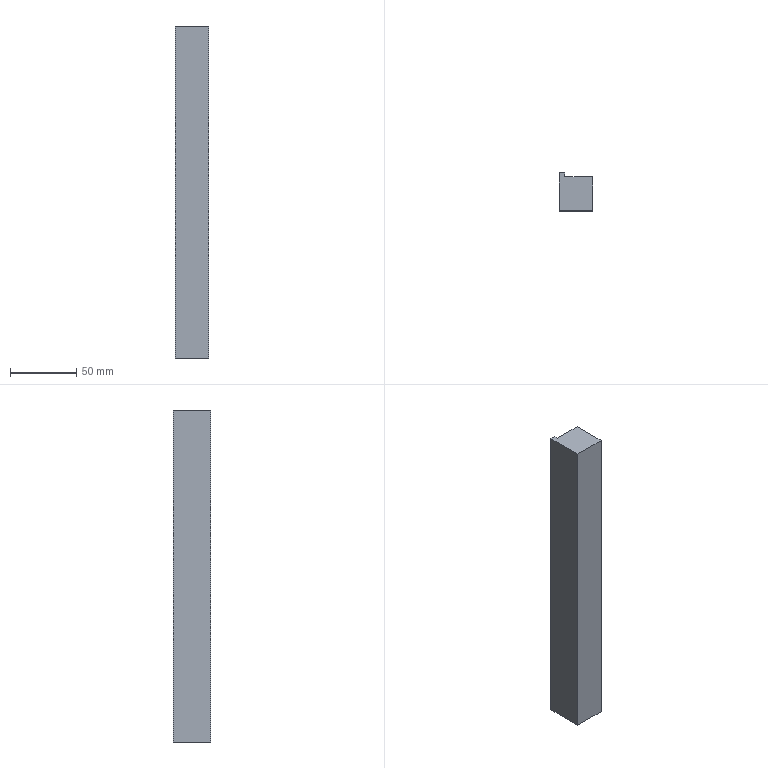Part | SolidWorks | features Extrusion 1 | 1 solid | 8 faces | box 25 x 28.5 x 250 mm | volume 162375 mm3 | plane 8
STEP:
#1=CARTESIAN_POINT('',(-10.,-15.5,0.));
#2=VERTEX_POINT('',#1);
#3=CARTESIAN_POINT('',(-10.,-12.5,0.));
#4=VERTEX_POINT('',#3);
#5=CARTESIAN_POINT('',(-10.,-15.5,0.));
#6=DIRECTION('',(0.,1.,0.));
#7=VECTOR('',#6,1000.);
#8=LINE('',#5,#7);
#9=EDGE_CURVE('',#2,#4,#8,.T.);
#10=ORIENTED_EDGE('',*,*,#9,.F.);
#11=CARTESIAN_POINT('',(-10.,-15.5,-250.));
#12=VERTEX_POINT('',#11);
#13=CARTESIAN_POINT('',(-10.,-15.5,-250.));
#14=DIRECTION('',(0.,0.,1.));
#15=VECTOR('',#14,1000.);
#16=LINE('',#13,#15);
#17=EDGE_CURVE('',#12,#2,#16,.T.);
#18=ORIENTED_EDGE('',*,*,#17,.F.);
#19=CARTESIAN_POINT('',(-10.,-12.5,-250.));
#20=VERTEX_POINT('',#19);
#21=CARTESIAN_POINT('',(-10.,-15.5,-250.));
#22=DIRECTION('',(0.,1.,0.));
#23=VECTOR('',#22,1000.);
#24=LINE('',#21,#23);
#25=EDGE_CURVE('',#12,#20,#24,.T.);
#26=ORIENTED_EDGE('',*,*,#25,.T.);
#27=CARTESIAN_POINT('',(-10.,-12.5,-250.));
#28=DIRECTION('',(0.,0.,1.));
#29=VECTOR('',#28,1000.);
#30=LINE('',#27,#29);
#31=EDGE_CURVE('',#20,#4,#30,.T.);
#32=ORIENTED_EDGE('',*,*,#31,.T.);
#33=EDGE_LOOP('',(#10,#18,#26,#32));
#34=FACE_OUTER_BOUND('',#33,.T.);
#35=CARTESIAN_POINT('',(-10.,-15.5,-250.));
#36=DIRECTION('',(1.,0.,0.));
#37=DIRECTION('',(0.,0.,-1.));
#38=AXIS2_PLACEMENT_3D('',#35,#36,#37);
#39=PLANE('',#38);
#40=ADVANCED_FACE('',(#34),#39,.T.);
#41=CARTESIAN_POINT('',(11.,-15.5,0.));
#42=VERTEX_POINT('',#41);
#43=CARTESIAN_POINT('',(11.,-15.5,0.));
#44=DIRECTION('',(-1.,0.,0.));
#45=VECTOR('',#44,1000.);
#46=LINE('',#43,#45);
#47=EDGE_CURVE('',#42,#2,#46,.T.);
#48=ORIENTED_EDGE('',*,*,#47,.F.);
#49=CARTESIAN_POINT('',(11.,-15.5,-250.));
#50=VERTEX_POINT('',#49);
#51=CARTESIAN_POINT('',(11.,-15.5,-250.));
#52=DIRECTION('',(0.,0.,1.));
#53=VECTOR('',#52,1000.);
#54=LINE('',#51,#53);
#55=EDGE_CURVE('',#50,#42,#54,.T.);
#56=ORIENTED_EDGE('',*,*,#55,.F.);
#57=CARTESIAN_POINT('',(11.,-15.5,-250.));
#58=DIRECTION('',(-1.,0.,0.));
#59=VECTOR('',#58,1000.);
#60=LINE('',#57,#59);
#61=EDGE_CURVE('',#50,#12,#60,.T.);
#62=ORIENTED_EDGE('',*,*,#61,.T.);
#63=ORIENTED_EDGE('',*,*,#17,.T.);
#64=EDGE_LOOP('',(#48,#56,#62,#63));
#65=FACE_OUTER_BOUND('',#64,.T.);
#66=CARTESIAN_POINT('',(11.,-15.5,-250.));
#67=DIRECTION('',(0.,1.,0.));
#68=DIRECTION('',(-1.,0.,0.));
#69=AXIS2_PLACEMENT_3D('',#66,#67,#68);
#70=PLANE('',#69);
#71=ADVANCED_FACE('',(#65),#70,.T.);
#72=CARTESIAN_POINT('',(11.,-41.,0.));
#73=VERTEX_POINT('',#72);
#74=CARTESIAN_POINT('',(11.,-41.,0.));
#75=DIRECTION('',(0.,1.,0.));
#76=VECTOR('',#75,1000.);
#77=LINE('',#74,#76);
#78=EDGE_CURVE('',#73,#42,#77,.T.);
#79=ORIENTED_EDGE('',*,*,#78,.F.);
#80=CARTESIAN_POINT('',(11.,-41.,-250.));
#81=VERTEX_POINT('',#80);
#82=CARTESIAN_POINT('',(11.,-41.,-250.));
#83=DIRECTION('',(0.,0.,1.));
#84=VECTOR('',#83,1000.);
#85=LINE('',#82,#84);
#86=EDGE_CURVE('',#81,#73,#85,.T.);
#87=ORIENTED_EDGE('',*,*,#86,.F.);
#88=CARTESIAN_POINT('',(11.,-41.,-250.));
#89=DIRECTION('',(0.,1.,0.));
#90=VECTOR('',#89,1000.);
#91=LINE('',#88,#90);
#92=EDGE_CURVE('',#81,#50,#91,.T.);
#93=ORIENTED_EDGE('',*,*,#92,.T.);
#94=ORIENTED_EDGE('',*,*,#55,.T.);
#95=EDGE_LOOP('',(#79,#87,#93,#94));
#96=FACE_OUTER_BOUND('',#95,.T.);
#97=CARTESIAN_POINT('',(11.,-41.,-250.));
#98=DIRECTION('',(1.,0.,0.));
#99=DIRECTION('',(0.,0.,-1.));
#100=AXIS2_PLACEMENT_3D('',#97,#98,#99);
#101=PLANE('',#100);
#102=ADVANCED_FACE('',(#96),#101,.T.);
#103=CARTESIAN_POINT('',(-14.,-41.,0.));
#104=VERTEX_POINT('',#103);
#105=CARTESIAN_POINT('',(-14.,-41.,0.));
#106=DIRECTION('',(1.,0.,0.));
#107=VECTOR('',#106,1000.);
#108=LINE('',#105,#107);
#109=EDGE_CURVE('',#104,#73,#108,.T.);
#110=ORIENTED_EDGE('',*,*,#109,.F.);
#111=CARTESIAN_POINT('',(-14.,-41.,-250.));
#112=VERTEX_POINT('',#111);
#113=CARTESIAN_POINT('',(-14.,-41.,-250.));
#114=DIRECTION('',(0.,0.,1.));
#115=VECTOR('',#114,1000.);
#116=LINE('',#113,#115);
#117=EDGE_CURVE('',#112,#104,#116,.T.);
#118=ORIENTED_EDGE('',*,*,#117,.F.);
#119=CARTESIAN_POINT('',(-14.,-41.,-250.));
#120=DIRECTION('',(1.,0.,0.));
#121=VECTOR('',#120,1000.);
#122=LINE('',#119,#121);
#123=EDGE_CURVE('',#112,#81,#122,.T.);
#124=ORIENTED_EDGE('',*,*,#123,.T.);
#125=ORIENTED_EDGE('',*,*,#86,.T.);
#126=EDGE_LOOP('',(#110,#118,#124,#125));
#127=FACE_OUTER_BOUND('',#126,.T.);
#128=CARTESIAN_POINT('',(-14.,-41.,-250.));
#129=DIRECTION('',(0.,-1.,0.));
#130=DIRECTION('',(0.,0.,-1.));
#131=AXIS2_PLACEMENT_3D('',#128,#129,#130);
#132=PLANE('',#131);
#133=ADVANCED_FACE('',(#127),#132,.T.);
#134=CARTESIAN_POINT('',(-14.,-12.5,0.));
#135=VERTEX_POINT('',#134);
#136=CARTESIAN_POINT('',(-14.,-12.5,0.));
#137=DIRECTION('',(0.,-1.,0.));
#138=VECTOR('',#137,1000.);
#139=LINE('',#136,#138);
#140=EDGE_CURVE('',#135,#104,#139,.T.);
#141=ORIENTED_EDGE('',*,*,#140,.F.);
#142=CARTESIAN_POINT('',(-14.,-12.5,-250.));
#143=VERTEX_POINT('',#142);
#144=CARTESIAN_POINT('',(-14.,-12.5,-250.));
#145=DIRECTION('',(0.,0.,1.));
#146=VECTOR('',#145,1000.);
#147=LINE('',#144,#146);
#148=EDGE_CURVE('',#143,#135,#147,.T.);
#149=ORIENTED_EDGE('',*,*,#148,.F.);
#150=CARTESIAN_POINT('',(-14.,-12.5,-250.));
#151=DIRECTION('',(0.,-1.,0.));
#152=VECTOR('',#151,1000.);
#153=LINE('',#150,#152);
#154=EDGE_CURVE('',#143,#112,#153,.T.);
#155=ORIENTED_EDGE('',*,*,#154,.T.);
#156=ORIENTED_EDGE('',*,*,#117,.T.);
#157=EDGE_LOOP('',(#141,#149,#155,#156));
#158=FACE_OUTER_BOUND('',#157,.T.);
#159=CARTESIAN_POINT('',(-14.,-12.5,-250.));
#160=DIRECTION('',(-1.,0.,0.));
#161=DIRECTION('',(0.,-1.,0.));
#162=AXIS2_PLACEMENT_3D('',#159,#160,#161);
#163=PLANE('',#162);
#164=ADVANCED_FACE('',(#158),#163,.T.);
#165=CARTESIAN_POINT('',(-10.,-12.5,0.));
#166=DIRECTION('',(-1.,0.,0.));
#167=VECTOR('',#166,1000.);
#168=LINE('',#165,#167);
#169=EDGE_CURVE('',#4,#135,#168,.T.);
#170=ORIENTED_EDGE('',*,*,#169,.F.);
#171=ORIENTED_EDGE('',*,*,#31,.F.);
#172=CARTESIAN_POINT('',(-10.,-12.5,-250.));
#173=DIRECTION('',(-1.,0.,0.));
#174=VECTOR('',#173,1000.);
#175=LINE('',#172,#174);
#176=EDGE_CURVE('',#20,#143,#175,.T.);
#177=ORIENTED_EDGE('',*,*,#176,.T.);
#178=ORIENTED_EDGE('',*,*,#148,.T.);
#179=EDGE_LOOP('',(#170,#171,#177,#178));
#180=FACE_OUTER_BOUND('',#179,.T.);
#181=CARTESIAN_POINT('',(-10.,-12.5,-250.));
#182=DIRECTION('',(0.,1.,0.));
#183=DIRECTION('',(0.,0.,1.));
#184=AXIS2_PLACEMENT_3D('',#181,#182,#183);
#185=PLANE('',#184);
#186=ADVANCED_FACE('',(#180),#185,.T.);
#187=ORIENTED_EDGE('',*,*,#25,.F.);
#188=ORIENTED_EDGE('',*,*,#61,.F.);
#189=ORIENTED_EDGE('',*,*,#92,.F.);
#190=ORIENTED_EDGE('',*,*,#123,.F.);
#191=ORIENTED_EDGE('',*,*,#154,.F.);
#192=ORIENTED_EDGE('',*,*,#176,.F.);
#193=EDGE_LOOP('',(#187,#188,#189,#190,#191,#192));
#194=FACE_OUTER_BOUND('',#193,.T.);
#195=CARTESIAN_POINT('',(0.,0.,-250.));
#196=DIRECTION('',(0.,0.,1.));
#197=DIRECTION('',(1.,0.,0.));
#198=AXIS2_PLACEMENT_3D('',#195,#196,#197);
#199=PLANE('',#198);
#200=ADVANCED_FACE('',(#194),#199,.F.);
#201=ORIENTED_EDGE('',*,*,#9,.T.);
#202=ORIENTED_EDGE('',*,*,#169,.T.);
#203=ORIENTED_EDGE('',*,*,#140,.T.);
#204=ORIENTED_EDGE('',*,*,#109,.T.);
#205=ORIENTED_EDGE('',*,*,#78,.T.);
#206=ORIENTED_EDGE('',*,*,#47,.T.);
#207=EDGE_LOOP('',(#201,#202,#203,#204,#205,#206));
#208=FACE_OUTER_BOUND('',#207,.T.);
#209=CARTESIAN_POINT('',(0.,0.,0.));
#210=DIRECTION('',(0.,0.,1.));
#211=DIRECTION('',(1.,0.,0.));
#212=AXIS2_PLACEMENT_3D('',#209,#210,#211);
#213=PLANE('',#212);
#214=ADVANCED_FACE('',(#208),#213,.T.);
#215=CLOSED_SHELL('',(#40,#71,#102,#133,#164,#186,#200,#214));
#216=MANIFOLD_SOLID_BREP('',#215);
#217=CARTESIAN_POINT('',(0.,0.,0.));
#218=DIRECTION('',(0.,0.,1.));
#219=DIRECTION('',(1.,0.,0.));
#220=AXIS2_PLACEMENT_3D('',#217,#218,#219);
#221=(LENGTH_UNIT()NAMED_UNIT(*)SI_UNIT(.MILLI.,.METRE.));
#222=UNCERTAINTY_MEASURE_WITH_UNIT(LENGTH_MEASURE(0.00001),#221,'','');
#223=(NAMED_UNIT(*)PLANE_ANGLE_UNIT()SI_UNIT($,.RADIAN.));
#224=(NAMED_UNIT(*)SI_UNIT($,.STERADIAN.)SOLID_ANGLE_UNIT());
#225=(GEOMETRIC_REPRESENTATION_CONTEXT(3)GLOBAL_UNCERTAINTY_ASSIGNED_CONTEXT((#222))GLOBAL_UNIT_ASSIGNED_CONTEXT((#221,#223,#224))REPRESENTATION_CONTEXT('',''));
#226=ADVANCED_BREP_SHAPE_REPRESENTATION('',(#216,#220),#225);